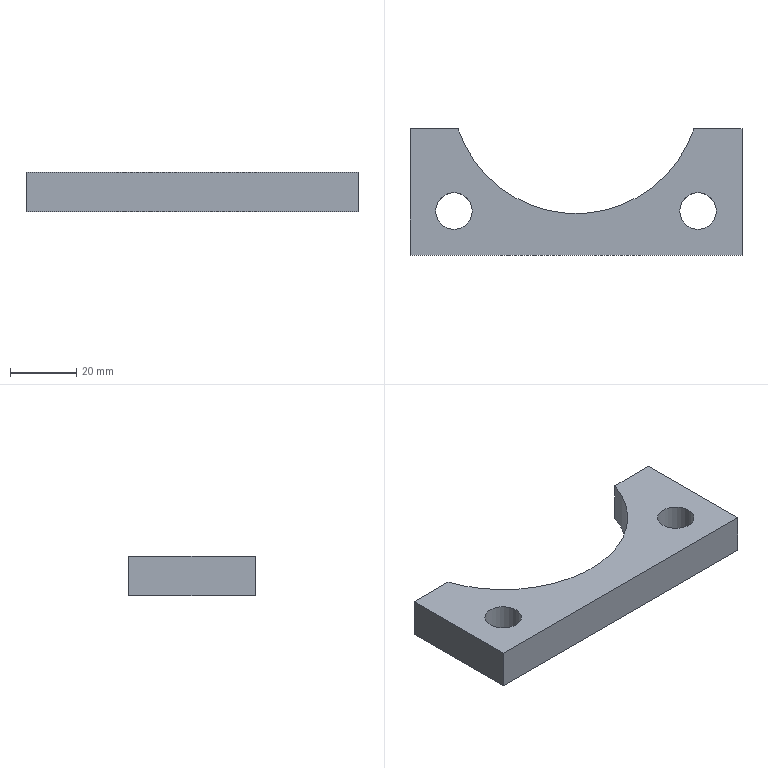Part | NX | features 3 2 | 1 solid | 10 faces | box 100 x 38 x 12 mm | volume 27425 mm3 | plane 7 | cylinder 3 | commonest cylinder face diameters 11 x2 75 x1
STEP:
#1=CARTESIAN_POINT('',(-1220.528,648.,-165.));
#2=VERTEX_POINT('',#1);
#3=CARTESIAN_POINT('',(-1220.528,648.,-153.));
#4=VERTEX_POINT('',#3);
#5=CARTESIAN_POINT('',(-1220.528,648.,-74.));
#6=DIRECTION('',(0.,0.,1.));
#7=VECTOR('',#6,1000.);
#8=LINE('',#5,#7);
#9=EDGE_CURVE('',#2,#4,#8,.T.);
#10=ORIENTED_EDGE('',*,*,#9,.F.);
#11=CARTESIAN_POINT('',(-1235.,648.,-165.));
#12=VERTEX_POINT('',#11);
#13=CARTESIAN_POINT('',(-1211.126,648.,-165.));
#14=DIRECTION('',(-1.,0.,0.));
#15=VECTOR('',#14,1000.);
#16=LINE('',#13,#15);
#17=EDGE_CURVE('',#2,#12,#16,.T.);
#18=ORIENTED_EDGE('',*,*,#17,.T.);
#19=CARTESIAN_POINT('',(-1235.,648.,-153.));
#20=VERTEX_POINT('',#19);
#21=CARTESIAN_POINT('',(-1235.,648.,-165.));
#22=DIRECTION('',(0.,0.,1.));
#23=VECTOR('',#22,1000.);
#24=LINE('',#21,#23);
#25=EDGE_CURVE('',#12,#20,#24,.T.);
#26=ORIENTED_EDGE('',*,*,#25,.T.);
#27=CARTESIAN_POINT('',(-1211.126,648.,-153.));
#28=DIRECTION('',(1.,0.,0.));
#29=VECTOR('',#28,1000.);
#30=LINE('',#27,#29);
#31=EDGE_CURVE('',#20,#4,#30,.T.);
#32=ORIENTED_EDGE('',*,*,#31,.T.);
#33=EDGE_LOOP('',(#10,#18,#26,#32));
#34=FACE_BOUND('',#33,.T.);
#35=CARTESIAN_POINT('',(-1227.5,648.,-165.));
#36=DIRECTION('',(0.,1.,0.));
#37=DIRECTION('',(-1.,0.,0.));
#38=AXIS2_PLACEMENT_3D('',#35,#36,#37);
#39=PLANE('',#38);
#40=ADVANCED_FACE('',(#34),#39,.T.);
#41=CARTESIAN_POINT('',(-1149.472,648.,-153.));
#42=VERTEX_POINT('',#41);
#43=CARTESIAN_POINT('',(-1149.472,648.,-165.));
#44=VERTEX_POINT('',#43);
#45=CARTESIAN_POINT('',(-1149.472,648.,-74.));
#46=DIRECTION('',(0.,0.,1.));
#47=VECTOR('',#46,1000.);
#48=LINE('',#45,#47);
#49=EDGE_CURVE('',#42,#44,#48,.F.);
#50=ORIENTED_EDGE('',*,*,#49,.F.);
#51=CARTESIAN_POINT('',(-1135.,648.,-153.));
#52=VERTEX_POINT('',#51);
#53=CARTESIAN_POINT('',(-1211.126,648.,-153.));
#54=DIRECTION('',(1.,0.,0.));
#55=VECTOR('',#54,1000.);
#56=LINE('',#53,#55);
#57=EDGE_CURVE('',#42,#52,#56,.T.);
#58=ORIENTED_EDGE('',*,*,#57,.T.);
#59=CARTESIAN_POINT('',(-1135.,648.,-165.));
#60=VERTEX_POINT('',#59);
#61=CARTESIAN_POINT('',(-1135.,648.,-165.));
#62=DIRECTION('',(0.,0.,1.));
#63=VECTOR('',#62,1000.);
#64=LINE('',#61,#63);
#65=EDGE_CURVE('',#60,#52,#64,.T.);
#66=ORIENTED_EDGE('',*,*,#65,.F.);
#67=CARTESIAN_POINT('',(-1211.126,648.,-165.));
#68=DIRECTION('',(-1.,0.,0.));
#69=VECTOR('',#68,1000.);
#70=LINE('',#67,#69);
#71=EDGE_CURVE('',#60,#44,#70,.T.);
#72=ORIENTED_EDGE('',*,*,#71,.T.);
#73=EDGE_LOOP('',(#50,#58,#66,#72));
#74=FACE_BOUND('',#73,.T.);
#75=CARTESIAN_POINT('',(-1227.5,648.,-165.));
#76=DIRECTION('',(0.,1.,0.));
#77=DIRECTION('',(-1.,0.,0.));
#78=AXIS2_PLACEMENT_3D('',#75,#76,#77);
#79=PLANE('',#78);
#80=ADVANCED_FACE('',(#74),#79,.T.);
#81=CARTESIAN_POINT('',(-1227.25,623.25,-165.));
#82=VERTEX_POINT('',#81);
#83=CARTESIAN_POINT('',(-1221.75,623.25,-165.));
#84=DIRECTION('',(0.,0.,1.));
#85=DIRECTION('',(-1.,0.,0.));
#86=AXIS2_PLACEMENT_3D('',#83,#84,#85);
#87=CIRCLE('',#86,5.5);
#88=EDGE_CURVE('',#82,#82,#87,.T.);
#89=ORIENTED_EDGE('',*,*,#88,.T.);
#90=EDGE_LOOP('',(#89));
#91=FACE_BOUND('',#90,.T.);
#92=CARTESIAN_POINT('',(-1153.75,623.25,-165.));
#93=VERTEX_POINT('',#92);
#94=CARTESIAN_POINT('',(-1148.25,623.25,-165.));
#95=DIRECTION('',(0.,0.,1.));
#96=DIRECTION('',(-1.,0.,0.));
#97=AXIS2_PLACEMENT_3D('',#94,#95,#96);
#98=CIRCLE('',#97,5.5);
#99=EDGE_CURVE('',#93,#93,#98,.T.);
#100=ORIENTED_EDGE('',*,*,#99,.T.);
#101=EDGE_LOOP('',(#100));
#102=FACE_BOUND('',#101,.T.);
#103=ORIENTED_EDGE('',*,*,#17,.F.);
#104=CARTESIAN_POINT('',(-1185.,660.,-165.));
#105=DIRECTION('',(0.,0.,-1.));
#106=DIRECTION('',(1.,0.,0.));
#107=AXIS2_PLACEMENT_3D('',#104,#105,#106);
#108=CIRCLE('',#107,37.5);
#109=EDGE_CURVE('',#2,#44,#108,.F.);
#110=ORIENTED_EDGE('',*,*,#109,.T.);
#111=ORIENTED_EDGE('',*,*,#71,.F.);
#112=CARTESIAN_POINT('',(-1135.,610.,-165.));
#113=VERTEX_POINT('',#112);
#114=CARTESIAN_POINT('',(-1135.,660.,-165.));
#115=DIRECTION('',(0.,1.,0.));
#116=VECTOR('',#115,1000.);
#117=LINE('',#114,#116);
#118=EDGE_CURVE('',#113,#60,#117,.T.);
#119=ORIENTED_EDGE('',*,*,#118,.F.);
#120=CARTESIAN_POINT('',(-1235.,610.,-165.));
#121=VERTEX_POINT('',#120);
#122=CARTESIAN_POINT('',(-1185.,610.,-165.));
#123=DIRECTION('',(1.,0.,0.));
#124=VECTOR('',#123,1000.);
#125=LINE('',#122,#124);
#126=EDGE_CURVE('',#121,#113,#125,.T.);
#127=ORIENTED_EDGE('',*,*,#126,.F.);
#128=CARTESIAN_POINT('',(-1235.,660.,-165.));
#129=DIRECTION('',(0.,-1.,0.));
#130=VECTOR('',#129,1000.);
#131=LINE('',#128,#130);
#132=EDGE_CURVE('',#12,#121,#131,.T.);
#133=ORIENTED_EDGE('',*,*,#132,.F.);
#134=EDGE_LOOP('',(#103,#110,#111,#119,#127,#133));
#135=FACE_BOUND('',#134,.T.);
#136=CARTESIAN_POINT('',(-1185.,660.,-165.));
#137=DIRECTION('',(0.,0.,1.));
#138=DIRECTION('',(1.,0.,0.));
#139=AXIS2_PLACEMENT_3D('',#136,#137,#138);
#140=PLANE('',#139);
#141=ADVANCED_FACE('',(#91,#102,#135),#140,.F.);
#142=CARTESIAN_POINT('',(-1235.,610.,-153.));
#143=VERTEX_POINT('',#142);
#144=CARTESIAN_POINT('',(-1235.,617.5,-153.));
#145=DIRECTION('',(0.,1.,0.));
#146=VECTOR('',#145,1000.);
#147=LINE('',#144,#146);
#148=EDGE_CURVE('',#143,#20,#147,.T.);
#149=ORIENTED_EDGE('',*,*,#148,.T.);
#150=ORIENTED_EDGE('',*,*,#25,.F.);
#151=ORIENTED_EDGE('',*,*,#132,.T.);
#152=CARTESIAN_POINT('',(-1235.,610.,-165.));
#153=DIRECTION('',(0.,0.,1.));
#154=VECTOR('',#153,1000.);
#155=LINE('',#152,#154);
#156=EDGE_CURVE('',#121,#143,#155,.T.);
#157=ORIENTED_EDGE('',*,*,#156,.T.);
#158=EDGE_LOOP('',(#149,#150,#151,#157));
#159=FACE_BOUND('',#158,.T.);
#160=CARTESIAN_POINT('',(-1235.,617.5,-165.));
#161=DIRECTION('',(-1.,0.,0.));
#162=DIRECTION('',(0.,0.,1.));
#163=AXIS2_PLACEMENT_3D('',#160,#161,#162);
#164=PLANE('',#163);
#165=ADVANCED_FACE('',(#159),#164,.T.);
#166=CARTESIAN_POINT('',(-1135.,610.,-153.));
#167=VERTEX_POINT('',#166);
#168=CARTESIAN_POINT('',(-1135.,648.,-153.));
#169=DIRECTION('',(0.,-1.,0.));
#170=VECTOR('',#169,1000.);
#171=LINE('',#168,#170);
#172=EDGE_CURVE('',#52,#167,#171,.T.);
#173=ORIENTED_EDGE('',*,*,#172,.T.);
#174=CARTESIAN_POINT('',(-1135.,610.,-165.));
#175=DIRECTION('',(0.,0.,1.));
#176=VECTOR('',#175,1000.);
#177=LINE('',#174,#176);
#178=EDGE_CURVE('',#113,#167,#177,.T.);
#179=ORIENTED_EDGE('',*,*,#178,.F.);
#180=ORIENTED_EDGE('',*,*,#118,.T.);
#181=ORIENTED_EDGE('',*,*,#65,.T.);
#182=EDGE_LOOP('',(#173,#179,#180,#181));
#183=FACE_BOUND('',#182,.T.);
#184=CARTESIAN_POINT('',(-1135.,648.,-165.));
#185=DIRECTION('',(1.,0.,0.));
#186=DIRECTION('',(0.,0.,-1.));
#187=AXIS2_PLACEMENT_3D('',#184,#185,#186);
#188=PLANE('',#187);
#189=ADVANCED_FACE('',(#183),#188,.T.);
#190=CARTESIAN_POINT('',(-1142.5,610.,-153.));
#191=DIRECTION('',(-1.,0.,0.));
#192=VECTOR('',#191,1000.);
#193=LINE('',#190,#192);
#194=EDGE_CURVE('',#167,#143,#193,.T.);
#195=ORIENTED_EDGE('',*,*,#194,.T.);
#196=ORIENTED_EDGE('',*,*,#156,.F.);
#197=ORIENTED_EDGE('',*,*,#126,.T.);
#198=ORIENTED_EDGE('',*,*,#178,.T.);
#199=EDGE_LOOP('',(#195,#196,#197,#198));
#200=FACE_BOUND('',#199,.T.);
#201=CARTESIAN_POINT('',(-1142.5,610.,-165.));
#202=DIRECTION('',(0.,-1.,0.));
#203=DIRECTION('',(1.,0.,0.));
#204=AXIS2_PLACEMENT_3D('',#201,#202,#203);
#205=PLANE('',#204);
#206=ADVANCED_FACE('',(#200),#205,.T.);
#207=CARTESIAN_POINT('',(-1185.,660.,-153.));
#208=DIRECTION('',(0.,0.,1.));
#209=DIRECTION('',(-1.,0.,0.));
#210=AXIS2_PLACEMENT_3D('',#207,#208,#209);
#211=CIRCLE('',#210,37.5);
#212=EDGE_CURVE('',#4,#42,#211,.T.);
#213=ORIENTED_EDGE('',*,*,#212,.F.);
#214=ORIENTED_EDGE('',*,*,#31,.F.);
#215=ORIENTED_EDGE('',*,*,#148,.F.);
#216=ORIENTED_EDGE('',*,*,#194,.F.);
#217=ORIENTED_EDGE('',*,*,#172,.F.);
#218=ORIENTED_EDGE('',*,*,#57,.F.);
#219=EDGE_LOOP('',(#213,#214,#215,#216,#217,#218));
#220=FACE_BOUND('',#219,.T.);
#221=CARTESIAN_POINT('',(-1216.25,623.25,-153.));
#222=VERTEX_POINT('',#221);
#223=CARTESIAN_POINT('',(-1221.75,623.25,-153.));
#224=DIRECTION('',(0.,0.,-1.));
#225=DIRECTION('',(1.,0.,0.));
#226=AXIS2_PLACEMENT_3D('',#223,#224,#225);
#227=CIRCLE('',#226,5.5);
#228=EDGE_CURVE('',#222,#222,#227,.T.);
#229=ORIENTED_EDGE('',*,*,#228,.T.);
#230=EDGE_LOOP('',(#229));
#231=FACE_BOUND('',#230,.T.);
#232=CARTESIAN_POINT('',(-1142.75,623.25,-153.));
#233=VERTEX_POINT('',#232);
#234=CARTESIAN_POINT('',(-1148.25,623.25,-153.));
#235=DIRECTION('',(0.,0.,-1.));
#236=DIRECTION('',(1.,0.,0.));
#237=AXIS2_PLACEMENT_3D('',#234,#235,#236);
#238=CIRCLE('',#237,5.5);
#239=EDGE_CURVE('',#233,#233,#238,.T.);
#240=ORIENTED_EDGE('',*,*,#239,.T.);
#241=EDGE_LOOP('',(#240));
#242=FACE_BOUND('',#241,.T.);
#243=CARTESIAN_POINT('',(-1185.,660.,-153.));
#244=DIRECTION('',(0.,0.,1.));
#245=DIRECTION('',(1.,0.,0.));
#246=AXIS2_PLACEMENT_3D('',#243,#244,#245);
#247=PLANE('',#246);
#248=ADVANCED_FACE('',(#220,#231,#242),#247,.T.);
#249=ORIENTED_EDGE('',*,*,#239,.F.);
#250=EDGE_LOOP('',(#249));
#251=FACE_BOUND('',#250,.T.);
#252=ORIENTED_EDGE('',*,*,#99,.F.);
#253=EDGE_LOOP('',(#252));
#254=FACE_BOUND('',#253,.T.);
#255=CARTESIAN_POINT('',(-1148.25,623.25,-153.));
#256=DIRECTION('',(0.,0.,-1.));
#257=DIRECTION('',(1.,0.,0.));
#258=AXIS2_PLACEMENT_3D('',#255,#256,#257);
#259=CYLINDRICAL_SURFACE('',#258,5.5);
#260=ADVANCED_FACE('',(#251,#254),#259,.F.);
#261=ORIENTED_EDGE('',*,*,#228,.F.);
#262=EDGE_LOOP('',(#261));
#263=FACE_BOUND('',#262,.T.);
#264=ORIENTED_EDGE('',*,*,#88,.F.);
#265=EDGE_LOOP('',(#264));
#266=FACE_BOUND('',#265,.T.);
#267=CARTESIAN_POINT('',(-1221.75,623.25,-153.));
#268=DIRECTION('',(0.,0.,-1.));
#269=DIRECTION('',(1.,0.,0.));
#270=AXIS2_PLACEMENT_3D('',#267,#268,#269);
#271=CYLINDRICAL_SURFACE('',#270,5.5);
#272=ADVANCED_FACE('',(#263,#266),#271,.F.);
#273=ORIENTED_EDGE('',*,*,#9,.T.);
#274=ORIENTED_EDGE('',*,*,#212,.T.);
#275=ORIENTED_EDGE('',*,*,#49,.T.);
#276=ORIENTED_EDGE('',*,*,#109,.F.);
#277=EDGE_LOOP('',(#273,#274,#275,#276));
#278=FACE_BOUND('',#277,.T.);
#279=CARTESIAN_POINT('',(-1185.,660.,-74.));
#280=DIRECTION('',(0.,0.,1.));
#281=DIRECTION('',(-1.,0.,0.));
#282=AXIS2_PLACEMENT_3D('',#279,#280,#281);
#283=CYLINDRICAL_SURFACE('',#282,37.5);
#284=ADVANCED_FACE('',(#278),#283,.F.);
#285=CLOSED_SHELL('',(#40,#80,#141,#165,#189,#206,#248,#260,#272,#284));
#286=MANIFOLD_SOLID_BREP('',#285);
#287=(LENGTH_UNIT()NAMED_UNIT(*)SI_UNIT(.MILLI.,.METRE.));
#288=UNCERTAINTY_MEASURE_WITH_UNIT(LENGTH_MEASURE(0.00001),#287,'','');
#289=(NAMED_UNIT(*)PLANE_ANGLE_UNIT()SI_UNIT($,.RADIAN.));
#290=(NAMED_UNIT(*)SI_UNIT($,.STERADIAN.)SOLID_ANGLE_UNIT());
#291=(GEOMETRIC_REPRESENTATION_CONTEXT(3)GLOBAL_UNCERTAINTY_ASSIGNED_CONTEXT((#288))GLOBAL_UNIT_ASSIGNED_CONTEXT((#287,#289,#290))REPRESENTATION_CONTEXT('',''));
#292=ADVANCED_BREP_SHAPE_REPRESENTATION('',(#286),#291);